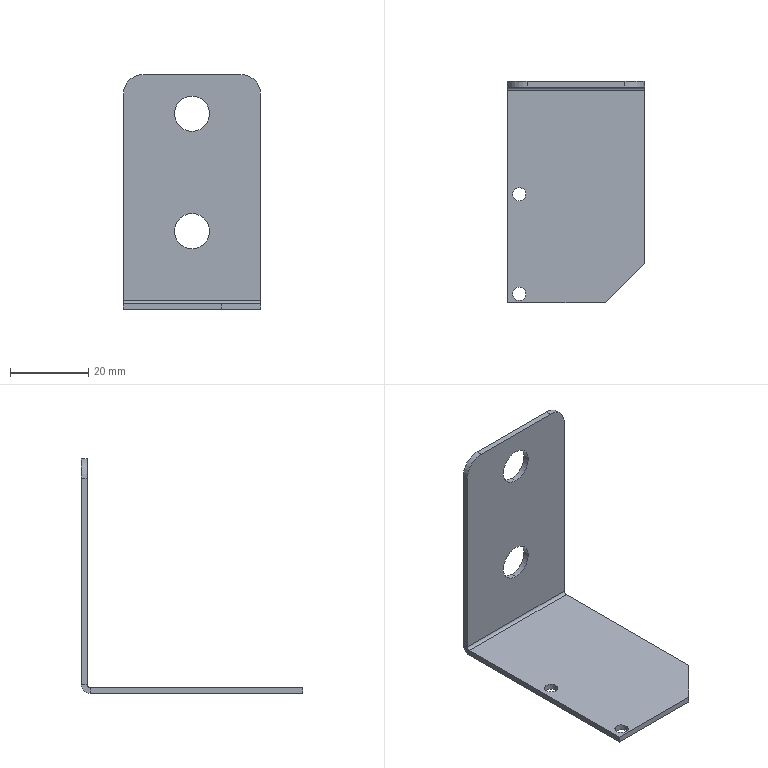Part | SolidWorks | features BaseBody 1 | 1 solid | 25 faces | box 35 x 56.5 x 60 mm | volume 5695 mm3 | plane 13 | cylinder 12 | commonest cylinder face diameters 3.4 x4 9 x4 10 x2 1.473 x1 4.473 x1
STEP:
#1=CARTESIAN_POINT('',(-16.2,-25.2,-1.5));
#2=VERTEX_POINT('',#1);
#3=CARTESIAN_POINT('',(-12.8,-25.2,-1.5));
#4=VERTEX_POINT('',#3);
#5=CARTESIAN_POINT('',(-14.5,-25.2,-1.5));
#6=DIRECTION('',(0.,0.,1.));
#7=DIRECTION('',(1.,0.,0.));
#8=AXIS2_PLACEMENT_3D('',#5,#6,#7);
#9=CIRCLE('',#8,1.7);
#10=EDGE_CURVE('',#2,#4,#9,.T.);
#11=ORIENTED_EDGE('',*,*,#10,.F.);
#12=CARTESIAN_POINT('',(-16.2,-25.2,0.));
#13=VERTEX_POINT('',#12);
#14=CARTESIAN_POINT('',(-16.2,-25.2,0.));
#15=DIRECTION('',(0.,0.,1.));
#16=VECTOR('',#15,1000.);
#17=LINE('',#14,#16);
#18=EDGE_CURVE('',#2,#13,#17,.T.);
#19=ORIENTED_EDGE('',*,*,#18,.T.);
#20=CARTESIAN_POINT('',(-12.8,-25.2,0.));
#21=VERTEX_POINT('',#20);
#22=CARTESIAN_POINT('',(-14.5,-25.2,0.));
#23=DIRECTION('',(0.,0.,1.));
#24=DIRECTION('',(1.,0.,0.));
#25=AXIS2_PLACEMENT_3D('',#22,#23,#24);
#26=CIRCLE('',#25,1.7);
#27=EDGE_CURVE('',#13,#21,#26,.T.);
#28=ORIENTED_EDGE('',*,*,#27,.T.);
#29=CARTESIAN_POINT('',(-12.8,-25.2,0.));
#30=DIRECTION('',(0.,0.,1.));
#31=VECTOR('',#30,1000.);
#32=LINE('',#29,#31);
#33=EDGE_CURVE('',#4,#21,#32,.T.);
#34=ORIENTED_EDGE('',*,*,#33,.F.);
#35=EDGE_LOOP('',(#11,#19,#28,#34));
#36=FACE_OUTER_BOUND('',#35,.T.);
#37=CARTESIAN_POINT('',(-14.5,-25.2,0.));
#38=DIRECTION('',(0.,0.,1.));
#39=DIRECTION('',(1.,0.,0.));
#40=AXIS2_PLACEMENT_3D('',#37,#38,#39);
#41=CYLINDRICAL_SURFACE('',#40,1.7);
#42=ADVANCED_FACE('',(#36),#41,.F.);
#43=CARTESIAN_POINT('',(-16.2,0.2,-1.5));
#44=VERTEX_POINT('',#43);
#45=CARTESIAN_POINT('',(-12.8,0.2,-1.5));
#46=VERTEX_POINT('',#45);
#47=CARTESIAN_POINT('',(-14.5,0.2,-1.5));
#48=DIRECTION('',(0.,0.,1.));
#49=DIRECTION('',(1.,0.,0.));
#50=AXIS2_PLACEMENT_3D('',#47,#48,#49);
#51=CIRCLE('',#50,1.7);
#52=EDGE_CURVE('',#44,#46,#51,.T.);
#53=ORIENTED_EDGE('',*,*,#52,.F.);
#54=CARTESIAN_POINT('',(-16.2,0.2,0.));
#55=VERTEX_POINT('',#54);
#56=CARTESIAN_POINT('',(-16.2,0.2,0.));
#57=DIRECTION('',(0.,0.,1.));
#58=VECTOR('',#57,1000.);
#59=LINE('',#56,#58);
#60=EDGE_CURVE('',#44,#55,#59,.T.);
#61=ORIENTED_EDGE('',*,*,#60,.T.);
#62=CARTESIAN_POINT('',(-12.8,0.2,0.));
#63=VERTEX_POINT('',#62);
#64=CARTESIAN_POINT('',(-14.5,0.2,0.));
#65=DIRECTION('',(0.,0.,1.));
#66=DIRECTION('',(1.,0.,0.));
#67=AXIS2_PLACEMENT_3D('',#64,#65,#66);
#68=CIRCLE('',#67,1.7);
#69=EDGE_CURVE('',#55,#63,#68,.T.);
#70=ORIENTED_EDGE('',*,*,#69,.T.);
#71=CARTESIAN_POINT('',(-12.8,0.2,0.));
#72=DIRECTION('',(0.,0.,1.));
#73=VECTOR('',#72,1000.);
#74=LINE('',#71,#73);
#75=EDGE_CURVE('',#46,#63,#74,.T.);
#76=ORIENTED_EDGE('',*,*,#75,.F.);
#77=EDGE_LOOP('',(#53,#61,#70,#76));
#78=FACE_OUTER_BOUND('',#77,.T.);
#79=CARTESIAN_POINT('',(-14.5,0.2,0.));
#80=DIRECTION('',(0.,0.,1.));
#81=DIRECTION('',(1.,0.,0.));
#82=AXIS2_PLACEMENT_3D('',#79,#80,#81);
#83=CYLINDRICAL_SURFACE('',#82,1.7);
#84=ADVANCED_FACE('',(#78),#83,.F.);
#85=CARTESIAN_POINT('',(0.,29.,53.));
#86=VERTEX_POINT('',#85);
#87=CARTESIAN_POINT('',(0.,29.,44.));
#88=VERTEX_POINT('',#87);
#89=CARTESIAN_POINT('',(0.,29.,48.5));
#90=DIRECTION('',(0.,-1.,0.));
#91=DIRECTION('',(0.,0.,-1.));
#92=AXIS2_PLACEMENT_3D('',#89,#90,#91);
#93=CIRCLE('',#92,4.5);
#94=EDGE_CURVE('',#86,#88,#93,.T.);
#95=ORIENTED_EDGE('',*,*,#94,.F.);
#96=CARTESIAN_POINT('',(0.,27.5,53.));
#97=VERTEX_POINT('',#96);
#98=CARTESIAN_POINT('',(0.,27.5,53.));
#99=DIRECTION('',(0.,-1.,0.));
#100=VECTOR('',#99,1000.);
#101=LINE('',#98,#100);
#102=EDGE_CURVE('',#86,#97,#101,.T.);
#103=ORIENTED_EDGE('',*,*,#102,.T.);
#104=CARTESIAN_POINT('',(0.,27.5,44.));
#105=VERTEX_POINT('',#104);
#106=CARTESIAN_POINT('',(0.,27.5,48.5));
#107=DIRECTION('',(0.,-1.,0.));
#108=DIRECTION('',(0.,0.,-1.));
#109=AXIS2_PLACEMENT_3D('',#106,#107,#108);
#110=CIRCLE('',#109,4.5);
#111=EDGE_CURVE('',#97,#105,#110,.T.);
#112=ORIENTED_EDGE('',*,*,#111,.T.);
#113=CARTESIAN_POINT('',(0.,27.5,44.));
#114=DIRECTION('',(0.,-1.,0.));
#115=VECTOR('',#114,1000.);
#116=LINE('',#113,#115);
#117=EDGE_CURVE('',#88,#105,#116,.T.);
#118=ORIENTED_EDGE('',*,*,#117,.F.);
#119=EDGE_LOOP('',(#95,#103,#112,#118));
#120=FACE_OUTER_BOUND('',#119,.T.);
#121=CARTESIAN_POINT('',(0.,27.5,48.5));
#122=DIRECTION('',(0.,-1.,0.));
#123=DIRECTION('',(0.,0.,-1.));
#124=AXIS2_PLACEMENT_3D('',#121,#122,#123);
#125=CYLINDRICAL_SURFACE('',#124,4.5);
#126=ADVANCED_FACE('',(#120),#125,.F.);
#127=CARTESIAN_POINT('',(0.,29.,23.));
#128=VERTEX_POINT('',#127);
#129=CARTESIAN_POINT('',(0.,29.,14.));
#130=VERTEX_POINT('',#129);
#131=CARTESIAN_POINT('',(0.,29.,18.5));
#132=DIRECTION('',(0.,-1.,0.));
#133=DIRECTION('',(0.,0.,-1.));
#134=AXIS2_PLACEMENT_3D('',#131,#132,#133);
#135=CIRCLE('',#134,4.5);
#136=EDGE_CURVE('',#128,#130,#135,.T.);
#137=ORIENTED_EDGE('',*,*,#136,.F.);
#138=CARTESIAN_POINT('',(0.,27.5,23.));
#139=VERTEX_POINT('',#138);
#140=CARTESIAN_POINT('',(0.,27.5,23.));
#141=DIRECTION('',(0.,-1.,0.));
#142=VECTOR('',#141,1000.);
#143=LINE('',#140,#142);
#144=EDGE_CURVE('',#128,#139,#143,.T.);
#145=ORIENTED_EDGE('',*,*,#144,.T.);
#146=CARTESIAN_POINT('',(0.,27.5,14.));
#147=VERTEX_POINT('',#146);
#148=CARTESIAN_POINT('',(0.,27.5,18.5));
#149=DIRECTION('',(0.,-1.,0.));
#150=DIRECTION('',(0.,0.,-1.));
#151=AXIS2_PLACEMENT_3D('',#148,#149,#150);
#152=CIRCLE('',#151,4.5);
#153=EDGE_CURVE('',#139,#147,#152,.T.);
#154=ORIENTED_EDGE('',*,*,#153,.T.);
#155=CARTESIAN_POINT('',(0.,27.5,14.));
#156=DIRECTION('',(0.,-1.,0.));
#157=VECTOR('',#156,1000.);
#158=LINE('',#155,#157);
#159=EDGE_CURVE('',#130,#147,#158,.T.);
#160=ORIENTED_EDGE('',*,*,#159,.F.);
#161=EDGE_LOOP('',(#137,#145,#154,#160));
#162=FACE_OUTER_BOUND('',#161,.T.);
#163=CARTESIAN_POINT('',(0.,27.5,18.5));
#164=DIRECTION('',(0.,-1.,0.));
#165=DIRECTION('',(0.,0.,-1.));
#166=AXIS2_PLACEMENT_3D('',#163,#164,#165);
#167=CYLINDRICAL_SURFACE('',#166,4.5);
#168=ADVANCED_FACE('',(#162),#167,.F.);
#169=CARTESIAN_POINT('',(-17.5,26.763,0.));
#170=VERTEX_POINT('',#169);
#171=CARTESIAN_POINT('',(-17.5,-27.5,0.));
#172=VERTEX_POINT('',#171);
#173=CARTESIAN_POINT('',(-17.5,27.5,0.));
#174=DIRECTION('',(0.,-1.,0.));
#175=VECTOR('',#174,1000.);
#176=LINE('',#173,#175);
#177=EDGE_CURVE('',#170,#172,#176,.T.);
#178=ORIENTED_EDGE('',*,*,#177,.F.);
#179=CARTESIAN_POINT('',(-17.5,26.763,-1.5));
#180=VERTEX_POINT('',#179);
#181=CARTESIAN_POINT('',(-17.5,26.763,0.));
#182=DIRECTION('',(0.,0.,-1.));
#183=VECTOR('',#182,1000.);
#184=LINE('',#181,#183);
#185=EDGE_CURVE('',#170,#180,#184,.T.);
#186=ORIENTED_EDGE('',*,*,#185,.T.);
#187=CARTESIAN_POINT('',(-17.5,-27.5,-1.5));
#188=VERTEX_POINT('',#187);
#189=CARTESIAN_POINT('',(-17.5,27.5,-1.5));
#190=DIRECTION('',(0.,-1.,0.));
#191=VECTOR('',#190,1000.);
#192=LINE('',#189,#191);
#193=EDGE_CURVE('',#180,#188,#192,.T.);
#194=ORIENTED_EDGE('',*,*,#193,.T.);
#195=CARTESIAN_POINT('',(-17.5,-27.5,-1.5));
#196=DIRECTION('',(0.,0.,1.));
#197=VECTOR('',#196,1000.);
#198=LINE('',#195,#197);
#199=EDGE_CURVE('',#188,#172,#198,.T.);
#200=ORIENTED_EDGE('',*,*,#199,.T.);
#201=EDGE_LOOP('',(#178,#186,#194,#200));
#202=FACE_OUTER_BOUND('',#201,.T.);
#203=CARTESIAN_POINT('',(-17.5,27.5,-1.5));
#204=DIRECTION('',(-1.,0.,0.));
#205=DIRECTION('',(0.,-1.,0.));
#206=AXIS2_PLACEMENT_3D('',#203,#204,#205);
#207=PLANE('',#206);
#208=ADVANCED_FACE('',(#202),#207,.T.);
#209=CARTESIAN_POINT('',(-14.5,-25.2,-1.5));
#210=DIRECTION('',(0.,0.,1.));
#211=DIRECTION('',(1.,0.,0.));
#212=AXIS2_PLACEMENT_3D('',#209,#210,#211);
#213=CIRCLE('',#212,1.7);
#214=EDGE_CURVE('',#4,#2,#213,.T.);
#215=ORIENTED_EDGE('',*,*,#214,.T.);
#216=ORIENTED_EDGE('',*,*,#10,.T.);
#217=EDGE_LOOP('',(#215,#216));
#218=FACE_BOUND('',#217,.T.);
#219=CARTESIAN_POINT('',(-14.5,0.2,-1.5));
#220=DIRECTION('',(0.,0.,1.));
#221=DIRECTION('',(1.,0.,0.));
#222=AXIS2_PLACEMENT_3D('',#219,#220,#221);
#223=CIRCLE('',#222,1.7);
#224=EDGE_CURVE('',#46,#44,#223,.T.);
#225=ORIENTED_EDGE('',*,*,#224,.T.);
#226=ORIENTED_EDGE('',*,*,#52,.T.);
#227=EDGE_LOOP('',(#225,#226));
#228=FACE_BOUND('',#227,.T.);
#229=CARTESIAN_POINT('',(17.5,-17.5,-1.5));
#230=VERTEX_POINT('',#229);
#231=CARTESIAN_POINT('',(17.5,26.763,-1.5));
#232=VERTEX_POINT('',#231);
#233=CARTESIAN_POINT('',(17.5,27.5,-1.5));
#234=DIRECTION('',(0.,1.,0.));
#235=VECTOR('',#234,1000.);
#236=LINE('',#233,#235);
#237=EDGE_CURVE('',#230,#232,#236,.T.);
#238=ORIENTED_EDGE('',*,*,#237,.F.);
#239=CARTESIAN_POINT('',(7.5,-27.5,-1.5));
#240=VERTEX_POINT('',#239);
#241=CARTESIAN_POINT('',(17.5,-17.5,-1.5));
#242=DIRECTION('',(-0.7071,-0.7071,0.));
#243=VECTOR('',#242,1000.);
#244=LINE('',#241,#243);
#245=EDGE_CURVE('',#230,#240,#244,.T.);
#246=ORIENTED_EDGE('',*,*,#245,.T.);
#247=CARTESIAN_POINT('',(17.5,-27.5,-1.5));
#248=DIRECTION('',(1.,0.,0.));
#249=VECTOR('',#248,1000.);
#250=LINE('',#247,#249);
#251=EDGE_CURVE('',#188,#240,#250,.T.);
#252=ORIENTED_EDGE('',*,*,#251,.F.);
#253=ORIENTED_EDGE('',*,*,#193,.F.);
#254=CARTESIAN_POINT('',(-17.5,26.763,-1.5));
#255=DIRECTION('',(1.,0.,0.));
#256=VECTOR('',#255,1000.);
#257=LINE('',#254,#256);
#258=EDGE_CURVE('',#180,#232,#257,.T.);
#259=ORIENTED_EDGE('',*,*,#258,.T.);
#260=EDGE_LOOP('',(#238,#246,#252,#253,#259));
#261=FACE_OUTER_BOUND('',#260,.T.);
#262=CARTESIAN_POINT('',(0.,0.,-1.5));
#263=DIRECTION('',(0.,0.,-1.));
#264=DIRECTION('',(-1.,0.,0.));
#265=AXIS2_PLACEMENT_3D('',#262,#263,#264);
#266=PLANE('',#265);
#267=ADVANCED_FACE('',(#218,#228,#261),#266,.T.);
#268=CARTESIAN_POINT('',(-14.5,-25.2,0.));
#269=DIRECTION('',(0.,0.,1.));
#270=DIRECTION('',(1.,0.,0.));
#271=AXIS2_PLACEMENT_3D('',#268,#269,#270);
#272=CIRCLE('',#271,1.7);
#273=EDGE_CURVE('',#21,#13,#272,.T.);
#274=ORIENTED_EDGE('',*,*,#273,.F.);
#275=ORIENTED_EDGE('',*,*,#27,.F.);
#276=EDGE_LOOP('',(#274,#275));
#277=FACE_BOUND('',#276,.T.);
#278=CARTESIAN_POINT('',(-14.5,0.2,0.));
#279=DIRECTION('',(0.,0.,1.));
#280=DIRECTION('',(1.,0.,0.));
#281=AXIS2_PLACEMENT_3D('',#278,#279,#280);
#282=CIRCLE('',#281,1.7);
#283=EDGE_CURVE('',#63,#55,#282,.T.);
#284=ORIENTED_EDGE('',*,*,#283,.F.);
#285=ORIENTED_EDGE('',*,*,#69,.F.);
#286=EDGE_LOOP('',(#284,#285));
#287=FACE_BOUND('',#286,.T.);
#288=CARTESIAN_POINT('',(7.5,-27.5,0.));
#289=VERTEX_POINT('',#288);
#290=CARTESIAN_POINT('',(17.5,-27.5,0.));
#291=DIRECTION('',(1.,0.,0.));
#292=VECTOR('',#291,1000.);
#293=LINE('',#290,#292);
#294=EDGE_CURVE('',#172,#289,#293,.T.);
#295=ORIENTED_EDGE('',*,*,#294,.T.);
#296=CARTESIAN_POINT('',(17.5,-17.5,0.));
#297=VERTEX_POINT('',#296);
#298=CARTESIAN_POINT('',(7.5,-27.5,0.));
#299=DIRECTION('',(0.7071,0.7071,0.));
#300=VECTOR('',#299,1000.);
#301=LINE('',#298,#300);
#302=EDGE_CURVE('',#289,#297,#301,.T.);
#303=ORIENTED_EDGE('',*,*,#302,.T.);
#304=CARTESIAN_POINT('',(17.5,26.763,0.));
#305=VERTEX_POINT('',#304);
#306=CARTESIAN_POINT('',(17.5,27.5,0.));
#307=DIRECTION('',(0.,1.,0.));
#308=VECTOR('',#307,1000.);
#309=LINE('',#306,#308);
#310=EDGE_CURVE('',#297,#305,#309,.T.);
#311=ORIENTED_EDGE('',*,*,#310,.T.);
#312=CARTESIAN_POINT('',(-17.5,26.763,0.));
#313=DIRECTION('',(1.,0.,0.));
#314=VECTOR('',#313,1000.);
#315=LINE('',#312,#314);
#316=EDGE_CURVE('',#170,#305,#315,.T.);
#317=ORIENTED_EDGE('',*,*,#316,.F.);
#318=ORIENTED_EDGE('',*,*,#177,.T.);
#319=EDGE_LOOP('',(#295,#303,#311,#317,#318));
#320=FACE_OUTER_BOUND('',#319,.T.);
#321=CARTESIAN_POINT('',(0.,0.,0.));
#322=DIRECTION('',(0.,0.,-1.));
#323=DIRECTION('',(-1.,0.,0.));
#324=AXIS2_PLACEMENT_3D('',#321,#322,#323);
#325=PLANE('',#324);
#326=ADVANCED_FACE('',(#277,#287,#320),#325,.F.);
#327=ORIENTED_EDGE('',*,*,#310,.F.);
#328=CARTESIAN_POINT('',(17.5,-17.5,-1.5));
#329=DIRECTION('',(0.,0.,-1.));
#330=VECTOR('',#329,1000.);
#331=LINE('',#328,#330);
#332=EDGE_CURVE('',#297,#230,#331,.T.);
#333=ORIENTED_EDGE('',*,*,#332,.T.);
#334=ORIENTED_EDGE('',*,*,#237,.T.);
#335=CARTESIAN_POINT('',(17.5,26.763,0.));
#336=DIRECTION('',(0.,0.,-1.));
#337=VECTOR('',#336,1000.);
#338=LINE('',#335,#337);
#339=EDGE_CURVE('',#305,#232,#338,.T.);
#340=ORIENTED_EDGE('',*,*,#339,.F.);
#341=EDGE_LOOP('',(#327,#333,#334,#340));
#342=FACE_OUTER_BOUND('',#341,.T.);
#343=CARTESIAN_POINT('',(17.5,27.5,-1.5));
#344=DIRECTION('',(1.,0.,0.));
#345=DIRECTION('',(0.,1.,0.));
#346=AXIS2_PLACEMENT_3D('',#343,#344,#345);
#347=PLANE('',#346);
#348=ADVANCED_FACE('',(#342),#347,.T.);
#349=ORIENTED_EDGE('',*,*,#251,.T.);
#350=CARTESIAN_POINT('',(7.5,-27.5,-1.5));
#351=DIRECTION('',(0.,0.,1.));
#352=VECTOR('',#351,1000.);
#353=LINE('',#350,#352);
#354=EDGE_CURVE('',#240,#289,#353,.T.);
#355=ORIENTED_EDGE('',*,*,#354,.T.);
#356=ORIENTED_EDGE('',*,*,#294,.F.);
#357=ORIENTED_EDGE('',*,*,#199,.F.);
#358=EDGE_LOOP('',(#349,#355,#356,#357));
#359=FACE_OUTER_BOUND('',#358,.T.);
#360=CARTESIAN_POINT('',(17.5,-27.5,-1.5));
#361=DIRECTION('',(0.,-1.,0.));
#362=DIRECTION('',(1.,0.,0.));
#363=AXIS2_PLACEMENT_3D('',#360,#361,#362);
#364=PLANE('',#363);
#365=ADVANCED_FACE('',(#359),#364,.T.);
#366=CARTESIAN_POINT('',(17.5,27.5,0.7366));
#367=VERTEX_POINT('',#366);
#368=CARTESIAN_POINT('',(17.5,29.,0.7366));
#369=VERTEX_POINT('',#368);
#370=CARTESIAN_POINT('',(17.5,27.5,0.7366));
#371=DIRECTION('',(0.,1.,0.));
#372=VECTOR('',#371,1000.);
#373=LINE('',#370,#372);
#374=EDGE_CURVE('',#367,#369,#373,.T.);
#375=ORIENTED_EDGE('',*,*,#374,.F.);
#376=CARTESIAN_POINT('',(17.5,26.763,0.7366));
#377=DIRECTION('',(1.,0.,0.));
#378=DIRECTION('',(0.,0.,1.));
#379=AXIS2_PLACEMENT_3D('',#376,#377,#378);
#380=CIRCLE('',#379,0.7366);
#381=EDGE_CURVE('',#305,#367,#380,.T.);
#382=ORIENTED_EDGE('',*,*,#381,.F.);
#383=ORIENTED_EDGE('',*,*,#339,.T.);
#384=CARTESIAN_POINT('',(17.5,26.763,0.7366));
#385=DIRECTION('',(1.,0.,0.));
#386=DIRECTION('',(0.,0.,1.));
#387=AXIS2_PLACEMENT_3D('',#384,#385,#386);
#388=CIRCLE('',#387,2.237);
#389=EDGE_CURVE('',#232,#369,#388,.T.);
#390=ORIENTED_EDGE('',*,*,#389,.T.);
#391=EDGE_LOOP('',(#375,#382,#383,#390));
#392=FACE_OUTER_BOUND('',#391,.T.);
#393=CARTESIAN_POINT('',(17.5,26.763,0.7366));
#394=DIRECTION('',(1.,0.,0.));
#395=DIRECTION('',(0.,0.,-1.));
#396=AXIS2_PLACEMENT_3D('',#393,#394,#395);
#397=PLANE('',#396);
#398=ADVANCED_FACE('',(#392),#397,.T.);
#399=CARTESIAN_POINT('',(-17.5,27.5,0.7366));
#400=VERTEX_POINT('',#399);
#401=CARTESIAN_POINT('',(-17.5,26.763,0.7366));
#402=DIRECTION('',(-1.,0.,0.));
#403=DIRECTION('',(0.,0.,1.));
#404=AXIS2_PLACEMENT_3D('',#401,#402,#403);
#405=CIRCLE('',#404,0.7366);
#406=EDGE_CURVE('',#400,#170,#405,.T.);
#407=ORIENTED_EDGE('',*,*,#406,.F.);
#408=CARTESIAN_POINT('',(-17.5,29.,0.7366));
#409=VERTEX_POINT('',#408);
#410=CARTESIAN_POINT('',(-17.5,27.5,0.7366));
#411=DIRECTION('',(0.,1.,0.));
#412=VECTOR('',#411,1000.);
#413=LINE('',#410,#412);
#414=EDGE_CURVE('',#400,#409,#413,.T.);
#415=ORIENTED_EDGE('',*,*,#414,.T.);
#416=CARTESIAN_POINT('',(-17.5,26.763,0.7366));
#417=DIRECTION('',(-1.,0.,0.));
#418=DIRECTION('',(0.,0.,1.));
#419=AXIS2_PLACEMENT_3D('',#416,#417,#418);
#420=CIRCLE('',#419,2.237);
#421=EDGE_CURVE('',#409,#180,#420,.T.);
#422=ORIENTED_EDGE('',*,*,#421,.T.);
#423=ORIENTED_EDGE('',*,*,#185,.F.);
#424=EDGE_LOOP('',(#407,#415,#422,#423));
#425=FACE_OUTER_BOUND('',#424,.T.);
#426=CARTESIAN_POINT('',(-17.5,26.763,0.7366));
#427=DIRECTION('',(1.,0.,0.));
#428=DIRECTION('',(0.,0.,-1.));
#429=AXIS2_PLACEMENT_3D('',#426,#427,#428);
#430=PLANE('',#429);
#431=ADVANCED_FACE('',(#425),#430,.F.);
#432=ORIENTED_EDGE('',*,*,#258,.F.);
#433=ORIENTED_EDGE('',*,*,#421,.F.);
#434=CARTESIAN_POINT('',(0.,29.,0.7366));
#435=DIRECTION('',(-1.,0.,0.));
#436=VECTOR('',#435,1000.);
#437=LINE('',#434,#436);
#438=EDGE_CURVE('',#369,#409,#437,.T.);
#439=ORIENTED_EDGE('',*,*,#438,.F.);
#440=ORIENTED_EDGE('',*,*,#389,.F.);
#441=EDGE_LOOP('',(#432,#433,#439,#440));
#442=FACE_OUTER_BOUND('',#441,.T.);
#443=CARTESIAN_POINT('',(-17.5,26.763,0.7366));
#444=DIRECTION('',(-1.,0.,0.));
#445=DIRECTION('',(0.,1.,0.));
#446=AXIS2_PLACEMENT_3D('',#443,#444,#445);
#447=CYLINDRICAL_SURFACE('',#446,2.237);
#448=ADVANCED_FACE('',(#442),#447,.T.);
#449=ORIENTED_EDGE('',*,*,#316,.T.);
#450=ORIENTED_EDGE('',*,*,#381,.T.);
#451=CARTESIAN_POINT('',(17.5,27.5,0.7366));
#452=DIRECTION('',(-1.,0.,0.));
#453=VECTOR('',#452,1000.);
#454=LINE('',#451,#453);
#455=EDGE_CURVE('',#367,#400,#454,.T.);
#456=ORIENTED_EDGE('',*,*,#455,.T.);
#457=ORIENTED_EDGE('',*,*,#406,.T.);
#458=EDGE_LOOP('',(#449,#450,#456,#457));
#459=FACE_OUTER_BOUND('',#458,.T.);
#460=CARTESIAN_POINT('',(-17.5,26.763,0.7366));
#461=DIRECTION('',(-1.,0.,0.));
#462=DIRECTION('',(0.,1.,0.));
#463=AXIS2_PLACEMENT_3D('',#460,#461,#462);
#464=CYLINDRICAL_SURFACE('',#463,0.7366);
#465=ADVANCED_FACE('',(#459),#464,.F.);
#466=CARTESIAN_POINT('',(-17.5,27.5,53.5));
#467=VERTEX_POINT('',#466);
#468=CARTESIAN_POINT('',(-17.5,27.5,0.));
#469=DIRECTION('',(0.,0.,-1.));
#470=VECTOR('',#469,1000.);
#471=LINE('',#468,#470);
#472=EDGE_CURVE('',#467,#400,#471,.T.);
#473=ORIENTED_EDGE('',*,*,#472,.F.);
#474=CARTESIAN_POINT('',(-17.5,29.,53.5));
#475=VERTEX_POINT('',#474);
#476=CARTESIAN_POINT('',(-17.5,29.,53.5));
#477=DIRECTION('',(0.,1.,0.));
#478=VECTOR('',#477,1000.);
#479=LINE('',#476,#478);
#480=EDGE_CURVE('',#467,#475,#479,.T.);
#481=ORIENTED_EDGE('',*,*,#480,.T.);
#482=CARTESIAN_POINT('',(-17.5,29.,0.));
#483=DIRECTION('',(0.,0.,-1.));
#484=VECTOR('',#483,1000.);
#485=LINE('',#482,#484);
#486=EDGE_CURVE('',#475,#409,#485,.T.);
#487=ORIENTED_EDGE('',*,*,#486,.T.);
#488=ORIENTED_EDGE('',*,*,#414,.F.);
#489=EDGE_LOOP('',(#473,#481,#487,#488));
#490=FACE_OUTER_BOUND('',#489,.T.);
#491=CARTESIAN_POINT('',(-17.5,29.,0.));
#492=DIRECTION('',(-1.,0.,0.));
#493=DIRECTION('',(0.,-1.,0.));
#494=AXIS2_PLACEMENT_3D('',#491,#492,#493);
#495=PLANE('',#494);
#496=ADVANCED_FACE('',(#490),#495,.T.);
#497=CARTESIAN_POINT('',(17.5,29.,53.5));
#498=VERTEX_POINT('',#497);
#499=CARTESIAN_POINT('',(17.5,29.,58.5));
#500=DIRECTION('',(0.,0.,1.));
#501=VECTOR('',#500,1000.);
#502=LINE('',#499,#501);
#503=EDGE_CURVE('',#369,#498,#502,.T.);
#504=ORIENTED_EDGE('',*,*,#503,.T.);
#505=CARTESIAN_POINT('',(17.5,27.5,53.5));
#506=VERTEX_POINT('',#505);
#507=CARTESIAN_POINT('',(17.5,29.,53.5));
#508=DIRECTION('',(0.,-1.,0.));
#509=VECTOR('',#508,1000.);
#510=LINE('',#507,#509);
#511=EDGE_CURVE('',#498,#506,#510,.T.);
#512=ORIENTED_EDGE('',*,*,#511,.T.);
#513=CARTESIAN_POINT('',(17.5,27.5,58.5));
#514=DIRECTION('',(0.,0.,1.));
#515=VECTOR('',#514,1000.);
#516=LINE('',#513,#515);
#517=EDGE_CURVE('',#367,#506,#516,.T.);
#518=ORIENTED_EDGE('',*,*,#517,.F.);
#519=ORIENTED_EDGE('',*,*,#374,.T.);
#520=EDGE_LOOP('',(#504,#512,#518,#519));
#521=FACE_OUTER_BOUND('',#520,.T.);
#522=CARTESIAN_POINT('',(17.5,29.,58.5));
#523=DIRECTION('',(1.,0.,0.));
#524=DIRECTION('',(0.,1.,0.));
#525=AXIS2_PLACEMENT_3D('',#522,#523,#524);
#526=PLANE('',#525);
#527=ADVANCED_FACE('',(#521),#526,.T.);
#528=CARTESIAN_POINT('',(0.,29.,48.5));
#529=DIRECTION('',(0.,-1.,0.));
#530=DIRECTION('',(0.,0.,-1.));
#531=AXIS2_PLACEMENT_3D('',#528,#529,#530);
#532=CIRCLE('',#531,4.5);
#533=EDGE_CURVE('',#88,#86,#532,.T.);
#534=ORIENTED_EDGE('',*,*,#533,.T.);
#535=ORIENTED_EDGE('',*,*,#94,.T.);
#536=EDGE_LOOP('',(#534,#535));
#537=FACE_BOUND('',#536,.T.);
#538=CARTESIAN_POINT('',(0.,29.,18.5));
#539=DIRECTION('',(0.,-1.,0.));
#540=DIRECTION('',(0.,0.,-1.));
#541=AXIS2_PLACEMENT_3D('',#538,#539,#540);
#542=CIRCLE('',#541,4.5);
#543=EDGE_CURVE('',#130,#128,#542,.T.);
#544=ORIENTED_EDGE('',*,*,#543,.T.);
#545=ORIENTED_EDGE('',*,*,#136,.T.);
#546=EDGE_LOOP('',(#544,#545));
#547=FACE_BOUND('',#546,.T.);
#548=ORIENTED_EDGE('',*,*,#486,.F.);
#549=CARTESIAN_POINT('',(-12.5,29.,58.5));
#550=VERTEX_POINT('',#549);
#551=CARTESIAN_POINT('',(-12.5,29.,53.5));
#552=DIRECTION('',(0.,1.,0.));
#553=DIRECTION('',(0.,0.,1.));
#554=AXIS2_PLACEMENT_3D('',#551,#552,#553);
#555=CIRCLE('',#554,5.);
#556=EDGE_CURVE('',#475,#550,#555,.T.);
#557=ORIENTED_EDGE('',*,*,#556,.T.);
#558=CARTESIAN_POINT('',(12.5,29.,58.5));
#559=VERTEX_POINT('',#558);
#560=CARTESIAN_POINT('',(-17.5,29.,58.5));
#561=DIRECTION('',(-1.,0.,0.));
#562=VECTOR('',#561,1000.);
#563=LINE('',#560,#562);
#564=EDGE_CURVE('',#559,#550,#563,.T.);
#565=ORIENTED_EDGE('',*,*,#564,.F.);
#566=CARTESIAN_POINT('',(12.5,29.,53.5));
#567=DIRECTION('',(0.,1.,0.));
#568=DIRECTION('',(0.,0.,1.));
#569=AXIS2_PLACEMENT_3D('',#566,#567,#568);
#570=CIRCLE('',#569,5.);
#571=EDGE_CURVE('',#559,#498,#570,.T.);
#572=ORIENTED_EDGE('',*,*,#571,.T.);
#573=ORIENTED_EDGE('',*,*,#503,.F.);
#574=ORIENTED_EDGE('',*,*,#438,.T.);
#575=EDGE_LOOP('',(#548,#557,#565,#572,#573,#574));
#576=FACE_OUTER_BOUND('',#575,.T.);
#577=CARTESIAN_POINT('',(0.,29.,0.));
#578=DIRECTION('',(0.,1.,0.));
#579=DIRECTION('',(0.,0.,1.));
#580=AXIS2_PLACEMENT_3D('',#577,#578,#579);
#581=PLANE('',#580);
#582=ADVANCED_FACE('',(#537,#547,#576),#581,.T.);
#583=CARTESIAN_POINT('',(0.,27.5,48.5));
#584=DIRECTION('',(0.,-1.,0.));
#585=DIRECTION('',(0.,0.,-1.));
#586=AXIS2_PLACEMENT_3D('',#583,#584,#585);
#587=CIRCLE('',#586,4.5);
#588=EDGE_CURVE('',#105,#97,#587,.T.);
#589=ORIENTED_EDGE('',*,*,#588,.F.);
#590=ORIENTED_EDGE('',*,*,#111,.F.);
#591=EDGE_LOOP('',(#589,#590));
#592=FACE_BOUND('',#591,.T.);
#593=CARTESIAN_POINT('',(0.,27.5,18.5));
#594=DIRECTION('',(0.,-1.,0.));
#595=DIRECTION('',(0.,0.,-1.));
#596=AXIS2_PLACEMENT_3D('',#593,#594,#595);
#597=CIRCLE('',#596,4.5);
#598=EDGE_CURVE('',#147,#139,#597,.T.);
#599=ORIENTED_EDGE('',*,*,#598,.F.);
#600=ORIENTED_EDGE('',*,*,#153,.F.);
#601=EDGE_LOOP('',(#599,#600));
#602=FACE_BOUND('',#601,.T.);
#603=CARTESIAN_POINT('',(12.5,27.5,58.5));
#604=VERTEX_POINT('',#603);
#605=CARTESIAN_POINT('',(-12.5,27.5,58.5));
#606=VERTEX_POINT('',#605);
#607=CARTESIAN_POINT('',(-17.5,27.5,58.5));
#608=DIRECTION('',(-1.,0.,0.));
#609=VECTOR('',#608,1000.);
#610=LINE('',#607,#609);
#611=EDGE_CURVE('',#604,#606,#610,.T.);
#612=ORIENTED_EDGE('',*,*,#611,.T.);
#613=CARTESIAN_POINT('',(-12.5,27.5,53.5));
#614=DIRECTION('',(0.,-1.,0.));
#615=DIRECTION('',(0.,0.,1.));
#616=AXIS2_PLACEMENT_3D('',#613,#614,#615);
#617=CIRCLE('',#616,5.);
#618=EDGE_CURVE('',#606,#467,#617,.T.);
#619=ORIENTED_EDGE('',*,*,#618,.T.);
#620=ORIENTED_EDGE('',*,*,#472,.T.);
#621=ORIENTED_EDGE('',*,*,#455,.F.);
#622=ORIENTED_EDGE('',*,*,#517,.T.);
#623=CARTESIAN_POINT('',(12.5,27.5,53.5));
#624=DIRECTION('',(0.,-1.,0.));
#625=DIRECTION('',(0.,0.,1.));
#626=AXIS2_PLACEMENT_3D('',#623,#624,#625);
#627=CIRCLE('',#626,5.);
#628=EDGE_CURVE('',#506,#604,#627,.T.);
#629=ORIENTED_EDGE('',*,*,#628,.T.);
#630=EDGE_LOOP('',(#612,#619,#620,#621,#622,#629));
#631=FACE_OUTER_BOUND('',#630,.T.);
#632=CARTESIAN_POINT('',(0.,27.5,0.));
#633=DIRECTION('',(0.,1.,0.));
#634=DIRECTION('',(0.,0.,1.));
#635=AXIS2_PLACEMENT_3D('',#632,#633,#634);
#636=PLANE('',#635);
#637=ADVANCED_FACE('',(#592,#602,#631),#636,.F.);
#638=ORIENTED_EDGE('',*,*,#564,.T.);
#639=CARTESIAN_POINT('',(-12.5,29.,58.5));
#640=DIRECTION('',(0.,-1.,0.));
#641=VECTOR('',#640,1000.);
#642=LINE('',#639,#641);
#643=EDGE_CURVE('',#550,#606,#642,.T.);
#644=ORIENTED_EDGE('',*,*,#643,.T.);
#645=ORIENTED_EDGE('',*,*,#611,.F.);
#646=CARTESIAN_POINT('',(12.5,29.,58.5));
#647=DIRECTION('',(0.,1.,0.));
#648=VECTOR('',#647,1000.);
#649=LINE('',#646,#648);
#650=EDGE_CURVE('',#604,#559,#649,.T.);
#651=ORIENTED_EDGE('',*,*,#650,.T.);
#652=EDGE_LOOP('',(#638,#644,#645,#651));
#653=FACE_OUTER_BOUND('',#652,.T.);
#654=CARTESIAN_POINT('',(-17.5,29.,58.5));
#655=DIRECTION('',(0.,0.,1.));
#656=DIRECTION('',(0.,-1.,0.));
#657=AXIS2_PLACEMENT_3D('',#654,#655,#656);
#658=PLANE('',#657);
#659=ADVANCED_FACE('',(#653),#658,.T.);
#660=ORIENTED_EDGE('',*,*,#556,.F.);
#661=ORIENTED_EDGE('',*,*,#480,.F.);
#662=ORIENTED_EDGE('',*,*,#618,.F.);
#663=ORIENTED_EDGE('',*,*,#643,.F.);
#664=EDGE_LOOP('',(#660,#661,#662,#663));
#665=FACE_OUTER_BOUND('',#664,.T.);
#666=CARTESIAN_POINT('',(-12.5,29.,53.5));
#667=DIRECTION('',(0.,-1.,0.));
#668=DIRECTION('',(0.,0.,-1.));
#669=AXIS2_PLACEMENT_3D('',#666,#667,#668);
#670=CYLINDRICAL_SURFACE('',#669,5.);
#671=ADVANCED_FACE('',(#665),#670,.T.);
#672=ORIENTED_EDGE('',*,*,#571,.F.);
#673=ORIENTED_EDGE('',*,*,#650,.F.);
#674=ORIENTED_EDGE('',*,*,#628,.F.);
#675=ORIENTED_EDGE('',*,*,#511,.F.);
#676=EDGE_LOOP('',(#672,#673,#674,#675));
#677=FACE_OUTER_BOUND('',#676,.T.);
#678=CARTESIAN_POINT('',(12.5,29.,53.5));
#679=DIRECTION('',(0.,-1.,0.));
#680=DIRECTION('',(0.,0.,-1.));
#681=AXIS2_PLACEMENT_3D('',#678,#679,#680);
#682=CYLINDRICAL_SURFACE('',#681,5.);
#683=ADVANCED_FACE('',(#677),#682,.T.);
#684=ORIENTED_EDGE('',*,*,#245,.F.);
#685=ORIENTED_EDGE('',*,*,#332,.F.);
#686=ORIENTED_EDGE('',*,*,#302,.F.);
#687=ORIENTED_EDGE('',*,*,#354,.F.);
#688=EDGE_LOOP('',(#684,#685,#686,#687));
#689=FACE_OUTER_BOUND('',#688,.T.);
#690=CARTESIAN_POINT('',(7.5,-27.5,-1.5));
#691=DIRECTION('',(-0.7071,0.7071,0.));
#692=DIRECTION('',(0.,0.,1.));
#693=AXIS2_PLACEMENT_3D('',#690,#691,#692);
#694=PLANE('',#693);
#695=ADVANCED_FACE('',(#689),#694,.F.);
#696=ORIENTED_EDGE('',*,*,#144,.F.);
#697=ORIENTED_EDGE('',*,*,#543,.F.);
#698=ORIENTED_EDGE('',*,*,#159,.T.);
#699=ORIENTED_EDGE('',*,*,#598,.T.);
#700=EDGE_LOOP('',(#696,#697,#698,#699));
#701=FACE_OUTER_BOUND('',#700,.T.);
#702=CARTESIAN_POINT('',(0.,27.5,18.5));
#703=DIRECTION('',(0.,-1.,0.));
#704=DIRECTION('',(0.,0.,-1.));
#705=AXIS2_PLACEMENT_3D('',#702,#703,#704);
#706=CYLINDRICAL_SURFACE('',#705,4.5);
#707=ADVANCED_FACE('',(#701),#706,.F.);
#708=ORIENTED_EDGE('',*,*,#102,.F.);
#709=ORIENTED_EDGE('',*,*,#533,.F.);
#710=ORIENTED_EDGE('',*,*,#117,.T.);
#711=ORIENTED_EDGE('',*,*,#588,.T.);
#712=EDGE_LOOP('',(#708,#709,#710,#711));
#713=FACE_OUTER_BOUND('',#712,.T.);
#714=CARTESIAN_POINT('',(0.,27.5,48.5));
#715=DIRECTION('',(0.,-1.,0.));
#716=DIRECTION('',(0.,0.,-1.));
#717=AXIS2_PLACEMENT_3D('',#714,#715,#716);
#718=CYLINDRICAL_SURFACE('',#717,4.5);
#719=ADVANCED_FACE('',(#713),#718,.F.);
#720=ORIENTED_EDGE('',*,*,#60,.F.);
#721=ORIENTED_EDGE('',*,*,#224,.F.);
#722=ORIENTED_EDGE('',*,*,#75,.T.);
#723=ORIENTED_EDGE('',*,*,#283,.T.);
#724=EDGE_LOOP('',(#720,#721,#722,#723));
#725=FACE_OUTER_BOUND('',#724,.T.);
#726=CARTESIAN_POINT('',(-14.5,0.2,0.));
#727=DIRECTION('',(0.,0.,1.));
#728=DIRECTION('',(1.,0.,0.));
#729=AXIS2_PLACEMENT_3D('',#726,#727,#728);
#730=CYLINDRICAL_SURFACE('',#729,1.7);
#731=ADVANCED_FACE('',(#725),#730,.F.);
#732=ORIENTED_EDGE('',*,*,#18,.F.);
#733=ORIENTED_EDGE('',*,*,#214,.F.);
#734=ORIENTED_EDGE('',*,*,#33,.T.);
#735=ORIENTED_EDGE('',*,*,#273,.T.);
#736=EDGE_LOOP('',(#732,#733,#734,#735));
#737=FACE_OUTER_BOUND('',#736,.T.);
#738=CARTESIAN_POINT('',(-14.5,-25.2,0.));
#739=DIRECTION('',(0.,0.,1.));
#740=DIRECTION('',(1.,0.,0.));
#741=AXIS2_PLACEMENT_3D('',#738,#739,#740);
#742=CYLINDRICAL_SURFACE('',#741,1.7);
#743=ADVANCED_FACE('',(#737),#742,.F.);
#744=CLOSED_SHELL('',(#42,#84,#126,#168,#208,#267,#326,#348,#365,#398,#431,#448,#465,#496,#527,#582,#637,#659,#671,#683,#695,#707,#719,#731,#743));
#745=MANIFOLD_SOLID_BREP('',#744);
#746=CARTESIAN_POINT('',(0.,0.,0.));
#747=DIRECTION('',(0.,0.,1.));
#748=DIRECTION('',(1.,0.,0.));
#749=AXIS2_PLACEMENT_3D('',#746,#747,#748);
#750=(LENGTH_UNIT()NAMED_UNIT(*)SI_UNIT(.MILLI.,.METRE.));
#751=UNCERTAINTY_MEASURE_WITH_UNIT(LENGTH_MEASURE(0.00001),#750,'','');
#752=(NAMED_UNIT(*)PLANE_ANGLE_UNIT()SI_UNIT($,.RADIAN.));
#753=(NAMED_UNIT(*)SI_UNIT($,.STERADIAN.)SOLID_ANGLE_UNIT());
#754=(GEOMETRIC_REPRESENTATION_CONTEXT(3)GLOBAL_UNCERTAINTY_ASSIGNED_CONTEXT((#751))GLOBAL_UNIT_ASSIGNED_CONTEXT((#750,#752,#753))REPRESENTATION_CONTEXT('',''));
#755=ADVANCED_BREP_SHAPE_REPRESENTATION('',(#745,#749),#754);